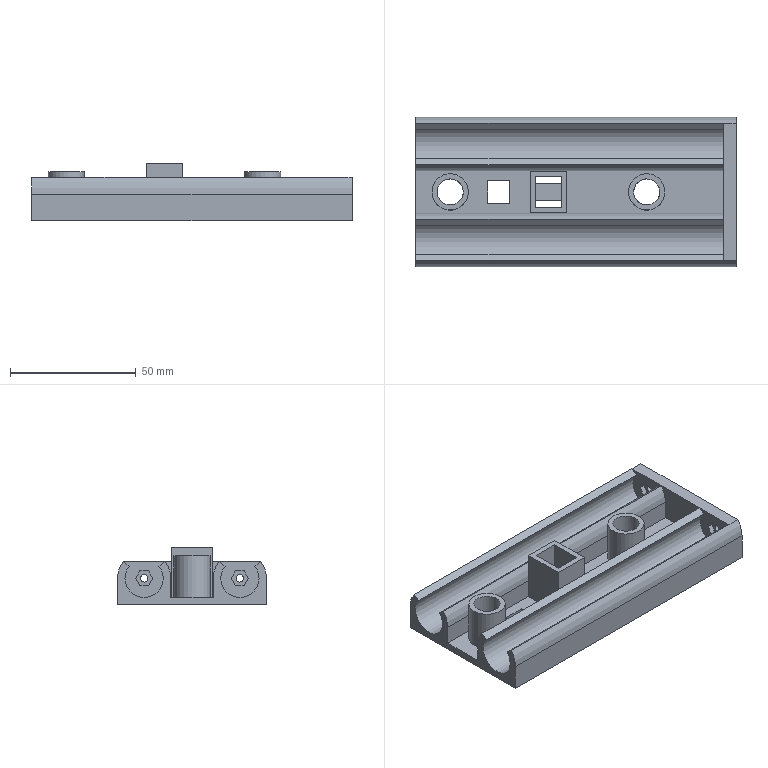Part | NX | features EXTRUDE 5, DATUM_CSYS 4, REPLACE_FACE 4, SKETCH 3, CHAMFER 1, OFFSET 1, UNITE 1 | 1 solid | 60 faces | box 127.15 x 59.2 x 23 mm | volume 56788 mm3 | plane 46 | cylinder 12 | cone 2 | commonest cylinder face diameters 21.2 x4 3 x2 10.4 x2 14.4 x2 15.2 x2